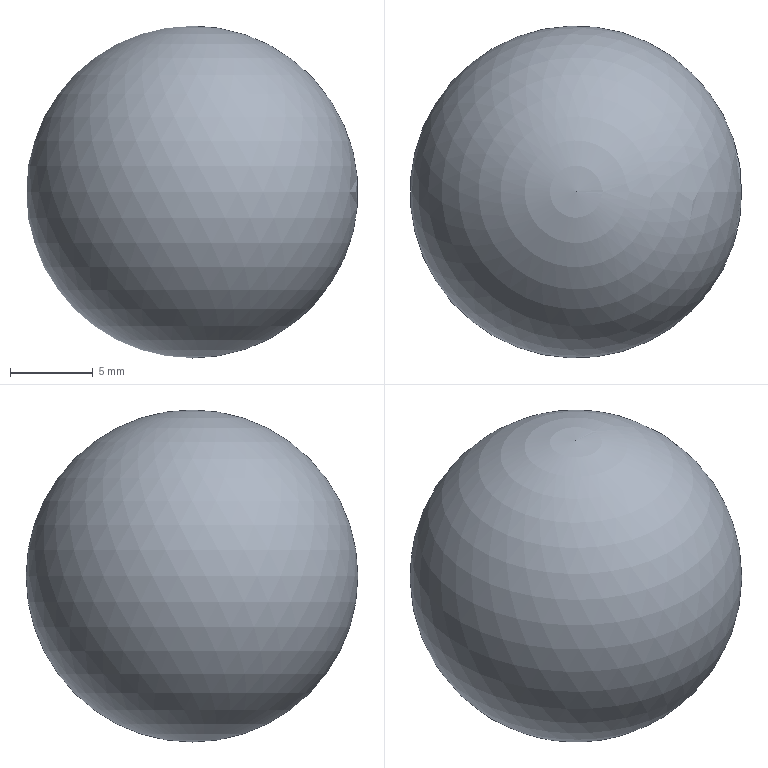Part | STEP file | solid 6 | 1 solid | 1 faces | box 20.1 x 20.1 x 20.1 mm | volume 4252 mm3 | sphere 1